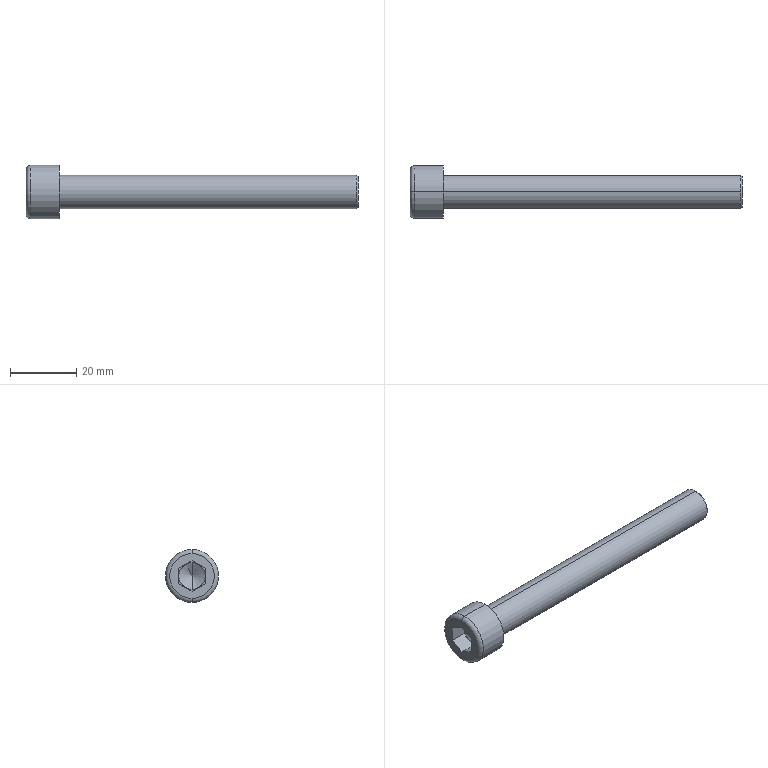Part | SolidWorks | features Fillet 2, RevCut 2, Boss 1, Chamfer 1, Cut 1, Extrusion 1, LPattern 1 | 1 solid | 25 faces | box 100 x 16 x 16 mm | volume 8745 mm3 | plane 15 | cone 4 | cylinder 4 | torus 2 | commonest cylinder face diameters 10 x2 16 x2
STEP:
#1=CARTESIAN_POINT('',(100.,0.,-4.6));
#2=VERTEX_POINT('',#1);
#3=CARTESIAN_POINT('',(100.,0.,4.6));
#4=VERTEX_POINT('',#3);
#5=CARTESIAN_POINT('',(100.,0.,0.));
#6=DIRECTION('',(1.,0.,0.));
#7=DIRECTION('',(0.,0.,-1.));
#8=AXIS2_PLACEMENT_3D('',#5,#6,#7);
#9=CIRCLE('',#8,4.6);
#10=EDGE_CURVE('',#2,#4,#9,.T.);
#11=ORIENTED_EDGE('',*,*,#10,.F.);
#12=CARTESIAN_POINT('',(99.6,0.,-5.));
#13=VERTEX_POINT('',#12);
#14=CARTESIAN_POINT('',(100.,0.,-4.6));
#15=DIRECTION('',(-0.7071,0.,-0.7071));
#16=VECTOR('',#15,1000.);
#17=LINE('',#14,#16);
#18=EDGE_CURVE('',#2,#13,#17,.T.);
#19=ORIENTED_EDGE('',*,*,#18,.T.);
#20=CARTESIAN_POINT('',(99.6,0.,5.));
#21=VERTEX_POINT('',#20);
#22=CARTESIAN_POINT('',(99.6,0.,0.));
#23=DIRECTION('',(-1.,0.,0.));
#24=DIRECTION('',(0.,0.,-1.));
#25=AXIS2_PLACEMENT_3D('',#22,#23,#24);
#26=CIRCLE('',#25,5.);
#27=EDGE_CURVE('',#21,#13,#26,.T.);
#28=ORIENTED_EDGE('',*,*,#27,.F.);
#29=CARTESIAN_POINT('',(100.,0.,4.6));
#30=DIRECTION('',(-0.7071,0.,0.7071));
#31=VECTOR('',#30,1000.);
#32=LINE('',#29,#31);
#33=EDGE_CURVE('',#4,#21,#32,.T.);
#34=ORIENTED_EDGE('',*,*,#33,.F.);
#35=EDGE_LOOP('',(#11,#19,#28,#34));
#36=FACE_OUTER_BOUND('',#35,.T.);
#37=CARTESIAN_POINT('',(100.,0.,0.));
#38=DIRECTION('',(-1.,0.,0.));
#39=DIRECTION('',(0.,0.,1.));
#40=AXIS2_PLACEMENT_3D('',#37,#38,#39);
#41=CONICAL_SURFACE('',#40,4.6,0.7854);
#42=ADVANCED_FACE('',(#36),#41,.T.);
#43=CARTESIAN_POINT('',(0.,0.,6.75));
#44=VERTEX_POINT('',#43);
#45=CARTESIAN_POINT('',(0.,0.,-6.75));
#46=VERTEX_POINT('',#45);
#47=CARTESIAN_POINT('',(0.,0.,0.));
#48=DIRECTION('',(-1.,0.,0.));
#49=DIRECTION('',(0.,0.,-1.));
#50=AXIS2_PLACEMENT_3D('',#47,#48,#49);
#51=CIRCLE('',#50,6.75);
#52=EDGE_CURVE('',#44,#46,#51,.T.);
#53=ORIENTED_EDGE('',*,*,#52,.F.);
#54=CARTESIAN_POINT('',(1.25,0.,8.));
#55=VERTEX_POINT('',#54);
#56=CARTESIAN_POINT('',(1.25,0.,6.75));
#57=DIRECTION('',(0.,1.,0.));
#58=DIRECTION('',(0.,0.,1.));
#59=AXIS2_PLACEMENT_3D('',#56,#57,#58);
#60=CIRCLE('',#59,1.25);
#61=EDGE_CURVE('',#44,#55,#60,.T.);
#62=ORIENTED_EDGE('',*,*,#61,.T.);
#63=CARTESIAN_POINT('',(1.25,0.,-8.));
#64=VERTEX_POINT('',#63);
#65=CARTESIAN_POINT('',(1.25,0.,0.));
#66=DIRECTION('',(1.,0.,0.));
#67=DIRECTION('',(0.,0.,-1.));
#68=AXIS2_PLACEMENT_3D('',#65,#66,#67);
#69=CIRCLE('',#68,8.);
#70=EDGE_CURVE('',#64,#55,#69,.T.);
#71=ORIENTED_EDGE('',*,*,#70,.F.);
#72=CARTESIAN_POINT('',(1.25,0.,-6.75));
#73=DIRECTION('',(0.,-1.,0.));
#74=DIRECTION('',(0.,0.,-1.));
#75=AXIS2_PLACEMENT_3D('',#72,#73,#74);
#76=CIRCLE('',#75,1.25);
#77=EDGE_CURVE('',#46,#64,#76,.T.);
#78=ORIENTED_EDGE('',*,*,#77,.F.);
#79=EDGE_LOOP('',(#53,#62,#71,#78));
#80=FACE_OUTER_BOUND('',#79,.T.);
#81=CARTESIAN_POINT('',(1.25,0.,0.));
#82=DIRECTION('',(1.,0.,0.));
#83=DIRECTION('',(0.,0.,-1.));
#84=AXIS2_PLACEMENT_3D('',#81,#82,#83);
#85=TOROIDAL_SURFACE('',#84,6.75,1.25);
#86=ADVANCED_FACE('',(#80),#85,.T.);
#87=CARTESIAN_POINT('',(7.309,0.,0.));
#88=VERTEX_POINT('',#87);
#89=CARTESIAN_POINT('',(5.,0.,4.));
#90=VERTEX_POINT('',#89);
#91=CARTESIAN_POINT('',(5.,0.,4.));
#92=DIRECTION('',(-0.5,0.,0.866));
#93=VECTOR('',#92,1000.);
#94=LINE('',#91,#93);
#95=EDGE_CURVE('',#88,#90,#94,.T.);
#96=ORIENTED_EDGE('',*,*,#95,.F.);
#97=CARTESIAN_POINT('',(5.,0.,-4.));
#98=VERTEX_POINT('',#97);
#99=CARTESIAN_POINT('',(5.,0.,-4.));
#100=DIRECTION('',(-0.5,0.,-0.866));
#101=VECTOR('',#100,1000.);
#102=LINE('',#99,#101);
#103=EDGE_CURVE('',#88,#98,#102,.T.);
#104=ORIENTED_EDGE('',*,*,#103,.T.);
#105=CARTESIAN_POINT('',(5.,-2.,-3.464));
#106=VERTEX_POINT('',#105);
#107=CARTESIAN_POINT('',(5.,0.,0.));
#108=DIRECTION('',(-1.,0.,0.));
#109=DIRECTION('',(0.,0.,-1.));
#110=AXIS2_PLACEMENT_3D('',#107,#108,#109);
#111=CIRCLE('',#110,4.);
#112=EDGE_CURVE('',#98,#106,#111,.T.);
#113=ORIENTED_EDGE('',*,*,#112,.T.);
#114=CARTESIAN_POINT('',(5.,-4.,0.));
#115=VERTEX_POINT('',#114);
#116=CARTESIAN_POINT('',(5.,0.,0.));
#117=DIRECTION('',(-1.,0.,0.));
#118=DIRECTION('',(0.,0.,-1.));
#119=AXIS2_PLACEMENT_3D('',#116,#117,#118);
#120=CIRCLE('',#119,4.);
#121=EDGE_CURVE('',#106,#115,#120,.T.);
#122=ORIENTED_EDGE('',*,*,#121,.T.);
#123=CARTESIAN_POINT('',(5.,-2.,3.464));
#124=VERTEX_POINT('',#123);
#125=CARTESIAN_POINT('',(5.,0.,0.));
#126=DIRECTION('',(-1.,0.,0.));
#127=DIRECTION('',(0.,0.,-1.));
#128=AXIS2_PLACEMENT_3D('',#125,#126,#127);
#129=CIRCLE('',#128,4.);
#130=EDGE_CURVE('',#115,#124,#129,.T.);
#131=ORIENTED_EDGE('',*,*,#130,.T.);
#132=CARTESIAN_POINT('',(5.,0.,0.));
#133=DIRECTION('',(-1.,0.,0.));
#134=DIRECTION('',(0.,0.,-1.));
#135=AXIS2_PLACEMENT_3D('',#132,#133,#134);
#136=CIRCLE('',#135,4.);
#137=EDGE_CURVE('',#124,#90,#136,.T.);
#138=ORIENTED_EDGE('',*,*,#137,.T.);
#139=EDGE_LOOP('',(#96,#104,#113,#122,#131,#138));
#140=FACE_OUTER_BOUND('',#139,.T.);
#141=CARTESIAN_POINT('',(5.,0.,0.));
#142=DIRECTION('',(-1.,0.,0.));
#143=DIRECTION('',(0.,0.,1.));
#144=AXIS2_PLACEMENT_3D('',#141,#142,#143);
#145=CONICAL_SURFACE('',#144,4.,1.047);
#146=ADVANCED_FACE('',(#140),#145,.F.);
#147=ORIENTED_EDGE('',*,*,#27,.T.);
#148=CARTESIAN_POINT('',(10.,0.,-5.));
#149=VERTEX_POINT('',#148);
#150=CARTESIAN_POINT('',(100.,0.,-5.));
#151=DIRECTION('',(-1.,0.,0.));
#152=VECTOR('',#151,1000.);
#153=LINE('',#150,#152);
#154=EDGE_CURVE('',#13,#149,#153,.T.);
#155=ORIENTED_EDGE('',*,*,#154,.T.);
#156=CARTESIAN_POINT('',(10.,0.,5.));
#157=VERTEX_POINT('',#156);
#158=CARTESIAN_POINT('',(10.,0.,0.));
#159=DIRECTION('',(1.,0.,0.));
#160=DIRECTION('',(0.,0.,-1.));
#161=AXIS2_PLACEMENT_3D('',#158,#159,#160);
#162=CIRCLE('',#161,5.);
#163=EDGE_CURVE('',#149,#157,#162,.T.);
#164=ORIENTED_EDGE('',*,*,#163,.T.);
#165=CARTESIAN_POINT('',(100.,0.,5.));
#166=DIRECTION('',(-1.,0.,0.));
#167=VECTOR('',#166,1000.);
#168=LINE('',#165,#167);
#169=EDGE_CURVE('',#21,#157,#168,.T.);
#170=ORIENTED_EDGE('',*,*,#169,.F.);
#171=EDGE_LOOP('',(#147,#155,#164,#170));
#172=FACE_OUTER_BOUND('',#171,.T.);
#173=CARTESIAN_POINT('',(100.,0.,0.));
#174=DIRECTION('',(-1.,0.,0.));
#175=DIRECTION('',(0.,0.,1.));
#176=AXIS2_PLACEMENT_3D('',#173,#174,#175);
#177=CYLINDRICAL_SURFACE('',#176,5.);
#178=ADVANCED_FACE('',(#172),#177,.T.);
#179=CARTESIAN_POINT('',(10.,0.,-8.));
#180=VERTEX_POINT('',#179);
#181=CARTESIAN_POINT('',(10.,0.,8.));
#182=VERTEX_POINT('',#181);
#183=CARTESIAN_POINT('',(10.,0.,0.));
#184=DIRECTION('',(1.,0.,0.));
#185=DIRECTION('',(0.,0.,-1.));
#186=AXIS2_PLACEMENT_3D('',#183,#184,#185);
#187=CIRCLE('',#186,8.);
#188=EDGE_CURVE('',#180,#182,#187,.T.);
#189=ORIENTED_EDGE('',*,*,#188,.F.);
#190=CARTESIAN_POINT('',(10.,0.,-8.));
#191=DIRECTION('',(-1.,0.,0.));
#192=VECTOR('',#191,1000.);
#193=LINE('',#190,#192);
#194=EDGE_CURVE('',#180,#64,#193,.T.);
#195=ORIENTED_EDGE('',*,*,#194,.T.);
#196=ORIENTED_EDGE('',*,*,#70,.T.);
#197=CARTESIAN_POINT('',(10.,0.,8.));
#198=DIRECTION('',(-1.,0.,0.));
#199=VECTOR('',#198,1000.);
#200=LINE('',#197,#199);
#201=EDGE_CURVE('',#182,#55,#200,.T.);
#202=ORIENTED_EDGE('',*,*,#201,.F.);
#203=EDGE_LOOP('',(#189,#195,#196,#202));
#204=FACE_OUTER_BOUND('',#203,.T.);
#205=CARTESIAN_POINT('',(10.,0.,0.));
#206=DIRECTION('',(-1.,0.,0.));
#207=DIRECTION('',(0.,0.,1.));
#208=AXIS2_PLACEMENT_3D('',#205,#206,#207);
#209=CYLINDRICAL_SURFACE('',#208,8.);
#210=ADVANCED_FACE('',(#204),#209,.T.);
#211=ORIENTED_EDGE('',*,*,#121,.F.);
#212=CARTESIAN_POINT('',(5.,-4.,-2.309));
#213=VERTEX_POINT('',#212);
#214=CARTESIAN_POINT('',(5.,-4.,-2.309));
#215=DIRECTION('',(0.,0.866,-0.5));
#216=VECTOR('',#215,1000.);
#217=LINE('',#214,#216);
#218=EDGE_CURVE('',#213,#106,#217,.T.);
#219=ORIENTED_EDGE('',*,*,#218,.F.);
#220=CARTESIAN_POINT('',(5.,-4.,2.309));
#221=DIRECTION('',(0.,0.,-1.));
#222=VECTOR('',#221,1000.);
#223=LINE('',#220,#222);
#224=EDGE_CURVE('',#115,#213,#223,.T.);
#225=ORIENTED_EDGE('',*,*,#224,.F.);
#226=EDGE_LOOP('',(#211,#219,#225));
#227=FACE_OUTER_BOUND('',#226,.T.);
#228=CARTESIAN_POINT('',(5.,0.,-4.619));
#229=DIRECTION('',(1.,0.,0.));
#230=DIRECTION('',(0.,0.,-1.));
#231=AXIS2_PLACEMENT_3D('',#228,#229,#230);
#232=PLANE('',#231);
#233=ADVANCED_FACE('',(#227),#232,.F.);
#234=ORIENTED_EDGE('',*,*,#130,.F.);
#235=CARTESIAN_POINT('',(5.,-4.,2.309));
#236=VERTEX_POINT('',#235);
#237=CARTESIAN_POINT('',(5.,-4.,2.309));
#238=DIRECTION('',(0.,0.,-1.));
#239=VECTOR('',#238,1000.);
#240=LINE('',#237,#239);
#241=EDGE_CURVE('',#236,#115,#240,.T.);
#242=ORIENTED_EDGE('',*,*,#241,.F.);
#243=CARTESIAN_POINT('',(5.,0.,4.619));
#244=DIRECTION('',(0.,-0.866,-0.5));
#245=VECTOR('',#244,1000.);
#246=LINE('',#243,#245);
#247=EDGE_CURVE('',#124,#236,#246,.T.);
#248=ORIENTED_EDGE('',*,*,#247,.F.);
#249=EDGE_LOOP('',(#234,#242,#248));
#250=FACE_OUTER_BOUND('',#249,.T.);
#251=CARTESIAN_POINT('',(5.,0.,-4.619));
#252=DIRECTION('',(1.,0.,0.));
#253=DIRECTION('',(0.,0.,-1.));
#254=AXIS2_PLACEMENT_3D('',#251,#252,#253);
#255=PLANE('',#254);
#256=ADVANCED_FACE('',(#250),#255,.F.);
#257=ORIENTED_EDGE('',*,*,#137,.F.);
#258=CARTESIAN_POINT('',(5.,0.,4.619));
#259=VERTEX_POINT('',#258);
#260=CARTESIAN_POINT('',(5.,0.,4.619));
#261=DIRECTION('',(0.,-0.866,-0.5));
#262=VECTOR('',#261,1000.);
#263=LINE('',#260,#262);
#264=EDGE_CURVE('',#259,#124,#263,.T.);
#265=ORIENTED_EDGE('',*,*,#264,.F.);
#266=CARTESIAN_POINT('',(5.,2.,3.464));
#267=VERTEX_POINT('',#266);
#268=CARTESIAN_POINT('',(5.,4.,2.309));
#269=DIRECTION('',(0.,-0.866,0.5));
#270=VECTOR('',#269,1000.);
#271=LINE('',#268,#270);
#272=EDGE_CURVE('',#267,#259,#271,.T.);
#273=ORIENTED_EDGE('',*,*,#272,.F.);
#274=CARTESIAN_POINT('',(5.,0.,0.));
#275=DIRECTION('',(-1.,0.,0.));
#276=DIRECTION('',(0.,0.,-1.));
#277=AXIS2_PLACEMENT_3D('',#274,#275,#276);
#278=CIRCLE('',#277,4.);
#279=EDGE_CURVE('',#90,#267,#278,.T.);
#280=ORIENTED_EDGE('',*,*,#279,.F.);
#281=EDGE_LOOP('',(#257,#265,#273,#280));
#282=FACE_OUTER_BOUND('',#281,.T.);
#283=CARTESIAN_POINT('',(5.,0.,-4.619));
#284=DIRECTION('',(1.,0.,0.));
#285=DIRECTION('',(0.,0.,-1.));
#286=AXIS2_PLACEMENT_3D('',#283,#284,#285);
#287=PLANE('',#286);
#288=ADVANCED_FACE('',(#282),#287,.F.);
#289=CARTESIAN_POINT('',(5.,4.,0.));
#290=VERTEX_POINT('',#289);
#291=CARTESIAN_POINT('',(5.,0.,0.));
#292=DIRECTION('',(-1.,0.,0.));
#293=DIRECTION('',(0.,0.,-1.));
#294=AXIS2_PLACEMENT_3D('',#291,#292,#293);
#295=CIRCLE('',#294,4.);
#296=EDGE_CURVE('',#267,#290,#295,.T.);
#297=ORIENTED_EDGE('',*,*,#296,.F.);
#298=CARTESIAN_POINT('',(5.,4.,2.309));
#299=VERTEX_POINT('',#298);
#300=CARTESIAN_POINT('',(5.,4.,2.309));
#301=DIRECTION('',(0.,-0.866,0.5));
#302=VECTOR('',#301,1000.);
#303=LINE('',#300,#302);
#304=EDGE_CURVE('',#299,#267,#303,.T.);
#305=ORIENTED_EDGE('',*,*,#304,.F.);
#306=CARTESIAN_POINT('',(5.,4.,-2.309));
#307=DIRECTION('',(0.,0.,1.));
#308=VECTOR('',#307,1000.);
#309=LINE('',#306,#308);
#310=EDGE_CURVE('',#290,#299,#309,.T.);
#311=ORIENTED_EDGE('',*,*,#310,.F.);
#312=EDGE_LOOP('',(#297,#305,#311));
#313=FACE_OUTER_BOUND('',#312,.T.);
#314=CARTESIAN_POINT('',(5.,0.,-4.619));
#315=DIRECTION('',(1.,0.,0.));
#316=DIRECTION('',(0.,0.,-1.));
#317=AXIS2_PLACEMENT_3D('',#314,#315,#316);
#318=PLANE('',#317);
#319=ADVANCED_FACE('',(#313),#318,.F.);
#320=CARTESIAN_POINT('',(5.,2.,-3.464));
#321=VERTEX_POINT('',#320);
#322=CARTESIAN_POINT('',(5.,0.,0.));
#323=DIRECTION('',(1.,0.,0.));
#324=DIRECTION('',(0.,0.,-1.));
#325=AXIS2_PLACEMENT_3D('',#322,#323,#324);
#326=CIRCLE('',#325,4.);
#327=EDGE_CURVE('',#321,#290,#326,.T.);
#328=ORIENTED_EDGE('',*,*,#327,.T.);
#329=CARTESIAN_POINT('',(5.,4.,-2.309));
#330=VERTEX_POINT('',#329);
#331=CARTESIAN_POINT('',(5.,4.,-2.309));
#332=DIRECTION('',(0.,0.,1.));
#333=VECTOR('',#332,1000.);
#334=LINE('',#331,#333);
#335=EDGE_CURVE('',#330,#290,#334,.T.);
#336=ORIENTED_EDGE('',*,*,#335,.F.);
#337=CARTESIAN_POINT('',(5.,0.,-4.619));
#338=DIRECTION('',(0.,0.866,0.5));
#339=VECTOR('',#338,1000.);
#340=LINE('',#337,#339);
#341=EDGE_CURVE('',#321,#330,#340,.T.);
#342=ORIENTED_EDGE('',*,*,#341,.F.);
#343=EDGE_LOOP('',(#328,#336,#342));
#344=FACE_OUTER_BOUND('',#343,.T.);
#345=CARTESIAN_POINT('',(5.,0.,-4.619));
#346=DIRECTION('',(1.,0.,0.));
#347=DIRECTION('',(0.,0.,-1.));
#348=AXIS2_PLACEMENT_3D('',#345,#346,#347);
#349=PLANE('',#348);
#350=ADVANCED_FACE('',(#344),#349,.F.);
#351=CARTESIAN_POINT('',(5.,0.,0.));
#352=DIRECTION('',(-1.,0.,0.));
#353=DIRECTION('',(0.,0.,-1.));
#354=AXIS2_PLACEMENT_3D('',#351,#352,#353);
#355=CIRCLE('',#354,4.);
#356=EDGE_CURVE('',#321,#98,#355,.T.);
#357=ORIENTED_EDGE('',*,*,#356,.F.);
#358=CARTESIAN_POINT('',(5.,0.,-4.619));
#359=VERTEX_POINT('',#358);
#360=CARTESIAN_POINT('',(5.,0.,-4.619));
#361=DIRECTION('',(0.,0.866,0.5));
#362=VECTOR('',#361,1000.);
#363=LINE('',#360,#362);
#364=EDGE_CURVE('',#359,#321,#363,.T.);
#365=ORIENTED_EDGE('',*,*,#364,.F.);
#366=CARTESIAN_POINT('',(5.,-4.,-2.309));
#367=DIRECTION('',(0.,0.866,-0.5));
#368=VECTOR('',#367,1000.);
#369=LINE('',#366,#368);
#370=EDGE_CURVE('',#106,#359,#369,.T.);
#371=ORIENTED_EDGE('',*,*,#370,.F.);
#372=ORIENTED_EDGE('',*,*,#112,.F.);
#373=EDGE_LOOP('',(#357,#365,#371,#372));
#374=FACE_OUTER_BOUND('',#373,.T.);
#375=CARTESIAN_POINT('',(5.,0.,-4.619));
#376=DIRECTION('',(1.,0.,0.));
#377=DIRECTION('',(0.,0.,-1.));
#378=AXIS2_PLACEMENT_3D('',#375,#376,#377);
#379=PLANE('',#378);
#380=ADVANCED_FACE('',(#374),#379,.F.);
#381=CARTESIAN_POINT('',(0.,0.,0.));
#382=DIRECTION('',(-1.,0.,0.));
#383=DIRECTION('',(0.,0.,-1.));
#384=AXIS2_PLACEMENT_3D('',#381,#382,#383);
#385=CIRCLE('',#384,6.75);
#386=EDGE_CURVE('',#46,#44,#385,.T.);
#387=ORIENTED_EDGE('',*,*,#386,.T.);
#388=ORIENTED_EDGE('',*,*,#52,.T.);
#389=EDGE_LOOP('',(#387,#388));
#390=FACE_OUTER_BOUND('',#389,.T.);
#391=CARTESIAN_POINT('',(0.,-4.,-2.309));
#392=VERTEX_POINT('',#391);
#393=CARTESIAN_POINT('',(0.,0.,-4.619));
#394=VERTEX_POINT('',#393);
#395=CARTESIAN_POINT('',(0.,-4.,-2.309));
#396=DIRECTION('',(0.,0.866,-0.5));
#397=VECTOR('',#396,1000.);
#398=LINE('',#395,#397);
#399=EDGE_CURVE('',#392,#394,#398,.T.);
#400=ORIENTED_EDGE('',*,*,#399,.T.);
#401=CARTESIAN_POINT('',(0.,4.,-2.309));
#402=VERTEX_POINT('',#401);
#403=CARTESIAN_POINT('',(0.,0.,-4.619));
#404=DIRECTION('',(0.,0.866,0.5));
#405=VECTOR('',#404,1000.);
#406=LINE('',#403,#405);
#407=EDGE_CURVE('',#394,#402,#406,.T.);
#408=ORIENTED_EDGE('',*,*,#407,.T.);
#409=CARTESIAN_POINT('',(0.,4.,2.309));
#410=VERTEX_POINT('',#409);
#411=CARTESIAN_POINT('',(0.,4.,-2.309));
#412=DIRECTION('',(0.,0.,1.));
#413=VECTOR('',#412,1000.);
#414=LINE('',#411,#413);
#415=EDGE_CURVE('',#402,#410,#414,.T.);
#416=ORIENTED_EDGE('',*,*,#415,.T.);
#417=CARTESIAN_POINT('',(0.,0.,4.619));
#418=VERTEX_POINT('',#417);
#419=CARTESIAN_POINT('',(0.,4.,2.309));
#420=DIRECTION('',(0.,-0.866,0.5));
#421=VECTOR('',#420,1000.);
#422=LINE('',#419,#421);
#423=EDGE_CURVE('',#410,#418,#422,.T.);
#424=ORIENTED_EDGE('',*,*,#423,.T.);
#425=CARTESIAN_POINT('',(0.,-4.,2.309));
#426=VERTEX_POINT('',#425);
#427=CARTESIAN_POINT('',(0.,0.,4.619));
#428=DIRECTION('',(0.,-0.866,-0.5));
#429=VECTOR('',#428,1000.);
#430=LINE('',#427,#429);
#431=EDGE_CURVE('',#418,#426,#430,.T.);
#432=ORIENTED_EDGE('',*,*,#431,.T.);
#433=CARTESIAN_POINT('',(0.,-4.,2.309));
#434=DIRECTION('',(0.,0.,-1.));
#435=VECTOR('',#434,1000.);
#436=LINE('',#433,#435);
#437=EDGE_CURVE('',#426,#392,#436,.T.);
#438=ORIENTED_EDGE('',*,*,#437,.T.);
#439=EDGE_LOOP('',(#400,#408,#416,#424,#432,#438));
#440=FACE_BOUND('',#439,.T.);
#441=CARTESIAN_POINT('',(0.,0.,0.));
#442=DIRECTION('',(1.,0.,0.));
#443=DIRECTION('',(0.,0.,-1.));
#444=AXIS2_PLACEMENT_3D('',#441,#442,#443);
#445=PLANE('',#444);
#446=ADVANCED_FACE('',(#390,#440),#445,.F.);
#447=CARTESIAN_POINT('',(10.,0.,0.));
#448=DIRECTION('',(1.,0.,0.));
#449=DIRECTION('',(0.,0.,-1.));
#450=AXIS2_PLACEMENT_3D('',#447,#448,#449);
#451=CIRCLE('',#450,8.);
#452=EDGE_CURVE('',#182,#180,#451,.T.);
#453=ORIENTED_EDGE('',*,*,#452,.T.);
#454=ORIENTED_EDGE('',*,*,#188,.T.);
#455=EDGE_LOOP('',(#453,#454));
#456=FACE_OUTER_BOUND('',#455,.T.);
#457=CARTESIAN_POINT('',(10.,0.,0.));
#458=DIRECTION('',(1.,0.,0.));
#459=DIRECTION('',(0.,0.,-1.));
#460=AXIS2_PLACEMENT_3D('',#457,#458,#459);
#461=CIRCLE('',#460,5.);
#462=EDGE_CURVE('',#157,#149,#461,.T.);
#463=ORIENTED_EDGE('',*,*,#462,.F.);
#464=ORIENTED_EDGE('',*,*,#163,.F.);
#465=EDGE_LOOP('',(#463,#464));
#466=FACE_BOUND('',#465,.T.);
#467=CARTESIAN_POINT('',(10.,0.,0.));
#468=DIRECTION('',(1.,0.,0.));
#469=DIRECTION('',(0.,0.,-1.));
#470=AXIS2_PLACEMENT_3D('',#467,#468,#469);
#471=PLANE('',#470);
#472=ADVANCED_FACE('',(#456,#466),#471,.T.);
#473=ORIENTED_EDGE('',*,*,#194,.F.);
#474=ORIENTED_EDGE('',*,*,#452,.F.);
#475=ORIENTED_EDGE('',*,*,#201,.T.);
#476=CARTESIAN_POINT('',(1.25,0.,0.));
#477=DIRECTION('',(1.,0.,0.));
#478=DIRECTION('',(0.,0.,-1.));
#479=AXIS2_PLACEMENT_3D('',#476,#477,#478);
#480=CIRCLE('',#479,8.);
#481=EDGE_CURVE('',#55,#64,#480,.T.);
#482=ORIENTED_EDGE('',*,*,#481,.T.);
#483=EDGE_LOOP('',(#473,#474,#475,#482));
#484=FACE_OUTER_BOUND('',#483,.T.);
#485=CARTESIAN_POINT('',(10.,0.,0.));
#486=DIRECTION('',(-1.,0.,0.));
#487=DIRECTION('',(0.,0.,1.));
#488=AXIS2_PLACEMENT_3D('',#485,#486,#487);
#489=CYLINDRICAL_SURFACE('',#488,8.);
#490=ADVANCED_FACE('',(#484),#489,.T.);
#491=ORIENTED_EDGE('',*,*,#154,.F.);
#492=CARTESIAN_POINT('',(99.6,0.,0.));
#493=DIRECTION('',(-1.,0.,0.));
#494=DIRECTION('',(0.,0.,-1.));
#495=AXIS2_PLACEMENT_3D('',#492,#493,#494);
#496=CIRCLE('',#495,5.);
#497=EDGE_CURVE('',#13,#21,#496,.T.);
#498=ORIENTED_EDGE('',*,*,#497,.T.);
#499=ORIENTED_EDGE('',*,*,#169,.T.);
#500=ORIENTED_EDGE('',*,*,#462,.T.);
#501=EDGE_LOOP('',(#491,#498,#499,#500));
#502=FACE_OUTER_BOUND('',#501,.T.);
#503=CARTESIAN_POINT('',(100.,0.,0.));
#504=DIRECTION('',(-1.,0.,0.));
#505=DIRECTION('',(0.,0.,1.));
#506=AXIS2_PLACEMENT_3D('',#503,#504,#505);
#507=CYLINDRICAL_SURFACE('',#506,5.);
#508=ADVANCED_FACE('',(#502),#507,.T.);
#509=CARTESIAN_POINT('',(100.,0.,0.));
#510=DIRECTION('',(1.,0.,0.));
#511=DIRECTION('',(0.,0.,-1.));
#512=AXIS2_PLACEMENT_3D('',#509,#510,#511);
#513=CIRCLE('',#512,4.6);
#514=EDGE_CURVE('',#4,#2,#513,.T.);
#515=ORIENTED_EDGE('',*,*,#514,.T.);
#516=ORIENTED_EDGE('',*,*,#10,.T.);
#517=EDGE_LOOP('',(#515,#516));
#518=FACE_OUTER_BOUND('',#517,.T.);
#519=CARTESIAN_POINT('',(100.,0.,0.));
#520=DIRECTION('',(1.,0.,0.));
#521=DIRECTION('',(0.,0.,-1.));
#522=AXIS2_PLACEMENT_3D('',#519,#520,#521);
#523=PLANE('',#522);
#524=ADVANCED_FACE('',(#518),#523,.T.);
#525=ORIENTED_EDGE('',*,*,#399,.F.);
#526=CARTESIAN_POINT('',(5.,-4.,-2.309));
#527=DIRECTION('',(-1.,0.,0.));
#528=VECTOR('',#527,1000.);
#529=LINE('',#526,#528);
#530=EDGE_CURVE('',#213,#392,#529,.T.);
#531=ORIENTED_EDGE('',*,*,#530,.F.);
#532=ORIENTED_EDGE('',*,*,#218,.T.);
#533=ORIENTED_EDGE('',*,*,#370,.T.);
#534=CARTESIAN_POINT('',(5.,0.,-4.619));
#535=DIRECTION('',(-1.,0.,0.));
#536=VECTOR('',#535,1000.);
#537=LINE('',#534,#536);
#538=EDGE_CURVE('',#359,#394,#537,.T.);
#539=ORIENTED_EDGE('',*,*,#538,.T.);
#540=EDGE_LOOP('',(#525,#531,#532,#533,#539));
#541=FACE_OUTER_BOUND('',#540,.T.);
#542=CARTESIAN_POINT('',(5.,-4.,-2.309));
#543=DIRECTION('',(0.,0.5,0.866));
#544=DIRECTION('',(0.,-0.866,0.5));
#545=AXIS2_PLACEMENT_3D('',#542,#543,#544);
#546=PLANE('',#545);
#547=ADVANCED_FACE('',(#541),#546,.T.);
#548=ORIENTED_EDGE('',*,*,#407,.F.);
#549=ORIENTED_EDGE('',*,*,#538,.F.);
#550=ORIENTED_EDGE('',*,*,#364,.T.);
#551=ORIENTED_EDGE('',*,*,#341,.T.);
#552=CARTESIAN_POINT('',(5.,4.,-2.309));
#553=DIRECTION('',(-1.,0.,0.));
#554=VECTOR('',#553,1000.);
#555=LINE('',#552,#554);
#556=EDGE_CURVE('',#330,#402,#555,.T.);
#557=ORIENTED_EDGE('',*,*,#556,.T.);
#558=EDGE_LOOP('',(#548,#549,#550,#551,#557));
#559=FACE_OUTER_BOUND('',#558,.T.);
#560=CARTESIAN_POINT('',(5.,0.,-4.619));
#561=DIRECTION('',(0.,-0.5,0.866));
#562=DIRECTION('',(0.,-0.866,-0.5));
#563=AXIS2_PLACEMENT_3D('',#560,#561,#562);
#564=PLANE('',#563);
#565=ADVANCED_FACE('',(#559),#564,.T.);
#566=ORIENTED_EDGE('',*,*,#415,.F.);
#567=ORIENTED_EDGE('',*,*,#556,.F.);
#568=ORIENTED_EDGE('',*,*,#335,.T.);
#569=ORIENTED_EDGE('',*,*,#310,.T.);
#570=CARTESIAN_POINT('',(5.,4.,2.309));
#571=DIRECTION('',(-1.,0.,0.));
#572=VECTOR('',#571,1000.);
#573=LINE('',#570,#572);
#574=EDGE_CURVE('',#299,#410,#573,.T.);
#575=ORIENTED_EDGE('',*,*,#574,.T.);
#576=EDGE_LOOP('',(#566,#567,#568,#569,#575));
#577=FACE_OUTER_BOUND('',#576,.T.);
#578=CARTESIAN_POINT('',(5.,4.,-2.309));
#579=DIRECTION('',(0.,-1.,0.));
#580=DIRECTION('',(0.,0.,-1.));
#581=AXIS2_PLACEMENT_3D('',#578,#579,#580);
#582=PLANE('',#581);
#583=ADVANCED_FACE('',(#577),#582,.T.);
#584=ORIENTED_EDGE('',*,*,#423,.F.);
#585=ORIENTED_EDGE('',*,*,#574,.F.);
#586=ORIENTED_EDGE('',*,*,#304,.T.);
#587=ORIENTED_EDGE('',*,*,#272,.T.);
#588=CARTESIAN_POINT('',(5.,0.,4.619));
#589=DIRECTION('',(-1.,0.,0.));
#590=VECTOR('',#589,1000.);
#591=LINE('',#588,#590);
#592=EDGE_CURVE('',#259,#418,#591,.T.);
#593=ORIENTED_EDGE('',*,*,#592,.T.);
#594=EDGE_LOOP('',(#584,#585,#586,#587,#593));
#595=FACE_OUTER_BOUND('',#594,.T.);
#596=CARTESIAN_POINT('',(5.,4.,2.309));
#597=DIRECTION('',(0.,-0.5,-0.866));
#598=DIRECTION('',(0.,0.866,-0.5));
#599=AXIS2_PLACEMENT_3D('',#596,#597,#598);
#600=PLANE('',#599);
#601=ADVANCED_FACE('',(#595),#600,.T.);
#602=ORIENTED_EDGE('',*,*,#431,.F.);
#603=ORIENTED_EDGE('',*,*,#592,.F.);
#604=ORIENTED_EDGE('',*,*,#264,.T.);
#605=ORIENTED_EDGE('',*,*,#247,.T.);
#606=CARTESIAN_POINT('',(5.,-4.,2.309));
#607=DIRECTION('',(-1.,0.,0.));
#608=VECTOR('',#607,1000.);
#609=LINE('',#606,#608);
#610=EDGE_CURVE('',#236,#426,#609,.T.);
#611=ORIENTED_EDGE('',*,*,#610,.T.);
#612=EDGE_LOOP('',(#602,#603,#604,#605,#611));
#613=FACE_OUTER_BOUND('',#612,.T.);
#614=CARTESIAN_POINT('',(5.,0.,4.619));
#615=DIRECTION('',(0.,0.5,-0.866));
#616=DIRECTION('',(0.,0.866,0.5));
#617=AXIS2_PLACEMENT_3D('',#614,#615,#616);
#618=PLANE('',#617);
#619=ADVANCED_FACE('',(#613),#618,.T.);
#620=ORIENTED_EDGE('',*,*,#437,.F.);
#621=ORIENTED_EDGE('',*,*,#610,.F.);
#622=ORIENTED_EDGE('',*,*,#241,.T.);
#623=ORIENTED_EDGE('',*,*,#224,.T.);
#624=ORIENTED_EDGE('',*,*,#530,.T.);
#625=EDGE_LOOP('',(#620,#621,#622,#623,#624));
#626=FACE_OUTER_BOUND('',#625,.T.);
#627=CARTESIAN_POINT('',(5.,-4.,2.309));
#628=DIRECTION('',(0.,1.,0.));
#629=DIRECTION('',(0.,0.,1.));
#630=AXIS2_PLACEMENT_3D('',#627,#628,#629);
#631=PLANE('',#630);
#632=ADVANCED_FACE('',(#626),#631,.T.);
#633=ORIENTED_EDGE('',*,*,#103,.F.);
#634=ORIENTED_EDGE('',*,*,#95,.T.);
#635=ORIENTED_EDGE('',*,*,#279,.T.);
#636=ORIENTED_EDGE('',*,*,#296,.T.);
#637=ORIENTED_EDGE('',*,*,#327,.F.);
#638=ORIENTED_EDGE('',*,*,#356,.T.);
#639=EDGE_LOOP('',(#633,#634,#635,#636,#637,#638));
#640=FACE_OUTER_BOUND('',#639,.T.);
#641=CARTESIAN_POINT('',(5.,0.,0.));
#642=DIRECTION('',(-1.,0.,0.));
#643=DIRECTION('',(0.,0.,1.));
#644=AXIS2_PLACEMENT_3D('',#641,#642,#643);
#645=CONICAL_SURFACE('',#644,4.,1.047);
#646=ADVANCED_FACE('',(#640),#645,.F.);
#647=ORIENTED_EDGE('',*,*,#61,.F.);
#648=ORIENTED_EDGE('',*,*,#386,.F.);
#649=ORIENTED_EDGE('',*,*,#77,.T.);
#650=ORIENTED_EDGE('',*,*,#481,.F.);
#651=EDGE_LOOP('',(#647,#648,#649,#650));
#652=FACE_OUTER_BOUND('',#651,.T.);
#653=CARTESIAN_POINT('',(1.25,0.,0.));
#654=DIRECTION('',(1.,0.,0.));
#655=DIRECTION('',(0.,0.,-1.));
#656=AXIS2_PLACEMENT_3D('',#653,#654,#655);
#657=TOROIDAL_SURFACE('',#656,6.75,1.25);
#658=ADVANCED_FACE('',(#652),#657,.T.);
#659=ORIENTED_EDGE('',*,*,#18,.F.);
#660=ORIENTED_EDGE('',*,*,#514,.F.);
#661=ORIENTED_EDGE('',*,*,#33,.T.);
#662=ORIENTED_EDGE('',*,*,#497,.F.);
#663=EDGE_LOOP('',(#659,#660,#661,#662));
#664=FACE_OUTER_BOUND('',#663,.T.);
#665=CARTESIAN_POINT('',(100.,0.,0.));
#666=DIRECTION('',(-1.,0.,0.));
#667=DIRECTION('',(0.,0.,1.));
#668=AXIS2_PLACEMENT_3D('',#665,#666,#667);
#669=CONICAL_SURFACE('',#668,4.6,0.7854);
#670=ADVANCED_FACE('',(#664),#669,.T.);
#671=CLOSED_SHELL('',(#42,#86,#146,#178,#210,#233,#256,#288,#319,#350,#380,#446,#472,#490,#508,#524,#547,#565,#583,#601,#619,#632,#646,#658,#670));
#672=MANIFOLD_SOLID_BREP('',#671);
#673=CARTESIAN_POINT('',(0.,0.,0.));
#674=DIRECTION('',(0.,0.,1.));
#675=DIRECTION('',(1.,0.,0.));
#676=AXIS2_PLACEMENT_3D('',#673,#674,#675);
#677=(LENGTH_UNIT()NAMED_UNIT(*)SI_UNIT(.MILLI.,.METRE.));
#678=UNCERTAINTY_MEASURE_WITH_UNIT(LENGTH_MEASURE(0.00001),#677,'','');
#679=(NAMED_UNIT(*)PLANE_ANGLE_UNIT()SI_UNIT($,.RADIAN.));
#680=(NAMED_UNIT(*)SI_UNIT($,.STERADIAN.)SOLID_ANGLE_UNIT());
#681=(GEOMETRIC_REPRESENTATION_CONTEXT(3)GLOBAL_UNCERTAINTY_ASSIGNED_CONTEXT((#678))GLOBAL_UNIT_ASSIGNED_CONTEXT((#677,#679,#680))REPRESENTATION_CONTEXT('',''));
#682=ADVANCED_BREP_SHAPE_REPRESENTATION('',(#672,#676),#681);